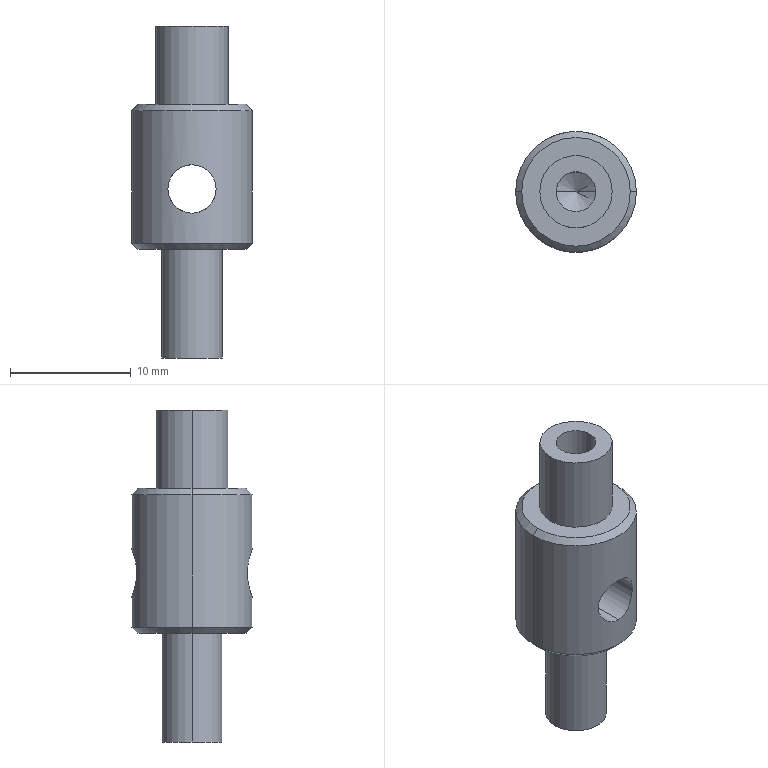Part | SolidWorks | features ICE 3, Chamfer 1, Extrusion 1, HoleWzd 1 | 1 solid | 20 faces | box 10 x 10 x 27.5 mm | volume 1083 mm3 | cylinder 10 | cone 6 | plane 4 | commonest cylinder face diameters 3.3 x2 4 x2 5 x2 6 x2 10 x2
STEP:
#1=CARTESIAN_POINT('',(-4.5,0.,0.));
#2=VERTEX_POINT('',#1);
#3=CARTESIAN_POINT('',(4.5,0.,0.));
#4=VERTEX_POINT('',#3);
#5=CARTESIAN_POINT('',(0.,0.,0.));
#6=DIRECTION('',(0.,0.,-1.));
#7=DIRECTION('',(1.,0.,0.));
#8=AXIS2_PLACEMENT_3D('',#5,#6,#7);
#9=CIRCLE('',#8,4.5);
#10=EDGE_CURVE('',#2,#4,#9,.T.);
#11=ORIENTED_EDGE('',*,*,#10,.F.);
#12=CARTESIAN_POINT('',(-5.,0.,0.5));
#13=VERTEX_POINT('',#12);
#14=CARTESIAN_POINT('',(-5.,0.,0.5));
#15=DIRECTION('',(-0.7071,0.,0.7071));
#16=VECTOR('',#15,1000.);
#17=LINE('',#14,#16);
#18=EDGE_CURVE('',#2,#13,#17,.T.);
#19=ORIENTED_EDGE('',*,*,#18,.T.);
#20=CARTESIAN_POINT('',(5.,0.,0.5));
#21=VERTEX_POINT('',#20);
#22=CARTESIAN_POINT('',(0.,0.,0.5));
#23=DIRECTION('',(0.,0.,1.));
#24=DIRECTION('',(1.,0.,0.));
#25=AXIS2_PLACEMENT_3D('',#22,#23,#24);
#26=CIRCLE('',#25,5.);
#27=EDGE_CURVE('',#21,#13,#26,.T.);
#28=ORIENTED_EDGE('',*,*,#27,.F.);
#29=CARTESIAN_POINT('',(5.,0.,0.5));
#30=DIRECTION('',(0.7071,0.,0.7071));
#31=VECTOR('',#30,1000.);
#32=LINE('',#29,#31);
#33=EDGE_CURVE('',#4,#21,#32,.T.);
#34=ORIENTED_EDGE('',*,*,#33,.F.);
#35=EDGE_LOOP('',(#11,#19,#28,#34));
#36=FACE_OUTER_BOUND('',#35,.T.);
#37=CARTESIAN_POINT('',(0.,0.,0.5));
#38=DIRECTION('',(0.,0.,1.));
#39=DIRECTION('',(1.,0.,0.));
#40=AXIS2_PLACEMENT_3D('',#37,#38,#39);
#41=CONICAL_SURFACE('',#40,5.,0.7854);
#42=ADVANCED_FACE('',(#36),#41,.T.);
#43=CARTESIAN_POINT('',(4.5,0.,12.));
#44=VERTEX_POINT('',#43);
#45=CARTESIAN_POINT('',(-4.5,0.,12.));
#46=VERTEX_POINT('',#45);
#47=CARTESIAN_POINT('',(0.,0.,12.));
#48=DIRECTION('',(0.,0.,1.));
#49=DIRECTION('',(1.,0.,0.));
#50=AXIS2_PLACEMENT_3D('',#47,#48,#49);
#51=CIRCLE('',#50,4.5);
#52=EDGE_CURVE('',#44,#46,#51,.T.);
#53=ORIENTED_EDGE('',*,*,#52,.F.);
#54=CARTESIAN_POINT('',(5.,0.,11.5));
#55=VERTEX_POINT('',#54);
#56=CARTESIAN_POINT('',(4.5,0.,12.));
#57=DIRECTION('',(0.7071,0.,-0.7071));
#58=VECTOR('',#57,1000.);
#59=LINE('',#56,#58);
#60=EDGE_CURVE('',#44,#55,#59,.T.);
#61=ORIENTED_EDGE('',*,*,#60,.T.);
#62=CARTESIAN_POINT('',(-5.,0.,11.5));
#63=VERTEX_POINT('',#62);
#64=CARTESIAN_POINT('',(0.,0.,11.5));
#65=DIRECTION('',(0.,0.,-1.));
#66=DIRECTION('',(1.,0.,0.));
#67=AXIS2_PLACEMENT_3D('',#64,#65,#66);
#68=CIRCLE('',#67,5.);
#69=EDGE_CURVE('',#63,#55,#68,.T.);
#70=ORIENTED_EDGE('',*,*,#69,.F.);
#71=CARTESIAN_POINT('',(-4.5,0.,12.));
#72=DIRECTION('',(-0.7071,0.,-0.7071));
#73=VECTOR('',#72,1000.);
#74=LINE('',#71,#73);
#75=EDGE_CURVE('',#46,#63,#74,.T.);
#76=ORIENTED_EDGE('',*,*,#75,.F.);
#77=EDGE_LOOP('',(#53,#61,#70,#76));
#78=FACE_OUTER_BOUND('',#77,.T.);
#79=CARTESIAN_POINT('',(0.,0.,12.));
#80=DIRECTION('',(0.,0.,-1.));
#81=DIRECTION('',(-1.,0.,0.));
#82=AXIS2_PLACEMENT_3D('',#79,#80,#81);
#83=CONICAL_SURFACE('',#82,4.5,0.7854);
#84=ADVANCED_FACE('',(#78),#83,.T.);
#85=CARTESIAN_POINT('',(0.,-5.,3.));
#86=VERTEX_POINT('',#85);
#87=CARTESIAN_POINT('',(0.,-5.,7.));
#88=VERTEX_POINT('',#87);
#89=CARTESIAN_POINT('',(0.,-5.,3.));
#90=CARTESIAN_POINT('',(-0.1316,-5.,3.));
#91=CARTESIAN_POINT('',(-0.2649,-4.995,3.013));
#92=CARTESIAN_POINT('',(-0.5241,-4.974,3.065));
#93=CARTESIAN_POINT('',(-0.6493,-4.959,3.104));
#94=CARTESIAN_POINT('',(-0.8912,-4.921,3.205));
#95=CARTESIAN_POINT('',(-1.008,-4.899,3.268));
#96=CARTESIAN_POINT('',(-1.223,-4.849,3.412));
#97=CARTESIAN_POINT('',(-1.323,-4.823,3.495));
#98=CARTESIAN_POINT('',(-1.507,-4.768,3.679));
#99=CARTESIAN_POINT('',(-1.589,-4.741,3.779));
#100=CARTESIAN_POINT('',(-1.733,-4.691,3.994));
#101=CARTESIAN_POINT('',(-1.796,-4.667,4.11));
#102=CARTESIAN_POINT('',(-1.896,-4.627,4.351));
#103=CARTESIAN_POINT('',(-1.935,-4.611,4.476));
#104=CARTESIAN_POINT('',(-1.987,-4.589,4.734));
#105=CARTESIAN_POINT('',(-2.,-4.583,4.868));
#106=CARTESIAN_POINT('',(-2.,-4.583,5.263));
#107=CARTESIAN_POINT('',(-1.946,-4.607,5.529));
#108=CARTESIAN_POINT('',(-1.796,-4.667,5.89));
#109=CARTESIAN_POINT('',(-1.733,-4.691,6.006));
#110=CARTESIAN_POINT('',(-1.589,-4.742,6.222));
#111=CARTESIAN_POINT('',(-1.507,-4.769,6.322));
#112=CARTESIAN_POINT('',(-1.323,-4.823,6.505));
#113=CARTESIAN_POINT('',(-1.222,-4.85,6.589));
#114=CARTESIAN_POINT('',(-1.007,-4.899,6.733));
#115=CARTESIAN_POINT('',(-0.8926,-4.921,6.795));
#116=CARTESIAN_POINT('',(-0.5273,-4.978,6.947));
#117=CARTESIAN_POINT('',(-0.2671,-5.,7.));
#118=CARTESIAN_POINT('',(0.,-5.,7.));
#119=B_SPLINE_CURVE_WITH_KNOTS('',3,(#89,#90,#91,#92,#93,#94,#95,#96,#97,#98,#99,#100,#101,#102,#103,#104,#105,#106,#107,#108,#109,#110,#111,#112,#113,#114,#115,#116,#117,#118),.UNSPECIFIED.,.F.,.F.,(4,2,2,2,2,2,2,2,2,2,2,2,2,2,4),(0.00632,0.006715,0.007109,0.007504,0.007899,0.008293,0.008688,0.009083,0.009478,0.01027,0.01066,0.01106,0.01145,0.01185,0.01264),.UNSPECIFIED.);
#120=EDGE_CURVE('',#86,#88,#119,.T.);
#121=ORIENTED_EDGE('',*,*,#120,.F.);
#122=CARTESIAN_POINT('',(0.,5.,3.));
#123=VERTEX_POINT('',#122);
#124=CARTESIAN_POINT('',(0.,-7.5,3.));
#125=DIRECTION('',(0.,1.,0.));
#126=VECTOR('',#125,1000.);
#127=LINE('',#124,#126);
#128=EDGE_CURVE('',#86,#123,#127,.T.);
#129=ORIENTED_EDGE('',*,*,#128,.T.);
#130=CARTESIAN_POINT('',(0.,5.,7.));
#131=VERTEX_POINT('',#130);
#132=CARTESIAN_POINT('',(0.,5.,7.));
#133=CARTESIAN_POINT('',(-0.1337,5.,7.));
#134=CARTESIAN_POINT('',(-0.2648,4.995,6.987));
#135=CARTESIAN_POINT('',(-0.5224,4.974,6.935));
#136=CARTESIAN_POINT('',(-0.6502,4.959,6.896));
#137=CARTESIAN_POINT('',(-0.8919,4.921,6.795));
#138=CARTESIAN_POINT('',(-1.006,4.899,6.733));
#139=CARTESIAN_POINT('',(-1.223,4.849,6.588));
#140=CARTESIAN_POINT('',(-1.324,4.822,6.505));
#141=CARTESIAN_POINT('',(-1.597,4.742,6.231));
#142=CARTESIAN_POINT('',(-1.746,4.687,6.01));
#143=CARTESIAN_POINT('',(-1.896,4.627,5.65));
#144=CARTESIAN_POINT('',(-1.935,4.61,5.523));
#145=CARTESIAN_POINT('',(-1.987,4.588,5.264));
#146=CARTESIAN_POINT('',(-2.,4.583,5.133));
#147=CARTESIAN_POINT('',(-2.,4.583,4.869));
#148=CARTESIAN_POINT('',(-1.987,4.588,4.735));
#149=CARTESIAN_POINT('',(-1.935,4.611,4.477));
#150=CARTESIAN_POINT('',(-1.897,4.627,4.352));
#151=CARTESIAN_POINT('',(-1.795,4.667,4.108));
#152=CARTESIAN_POINT('',(-1.733,4.691,3.994));
#153=CARTESIAN_POINT('',(-1.589,4.741,3.778));
#154=CARTESIAN_POINT('',(-1.505,4.769,3.677));
#155=CARTESIAN_POINT('',(-1.322,4.823,3.494));
#156=CARTESIAN_POINT('',(-1.223,4.85,3.412));
#157=CARTESIAN_POINT('',(-1.006,4.899,3.267));
#158=CARTESIAN_POINT('',(-0.8898,4.922,3.204));
#159=CARTESIAN_POINT('',(-0.5291,4.978,3.054));
#160=CARTESIAN_POINT('',(-0.2633,5.,3.));
#161=CARTESIAN_POINT('',(0.,5.,3.));
#162=B_SPLINE_CURVE_WITH_KNOTS('',3,(#132,#133,#134,#135,#136,#137,#138,#139,#140,#141,#142,#143,#144,#145,#146,#147,#148,#149,#150,#151,#152,#153,#154,#155,#156,#157,#158,#159,#160,#161),.UNSPECIFIED.,.F.,.F.,(4,2,2,2,2,2,2,2,2,2,2,2,2,2,4),(0.,0.000395,0.00079,0.001185,0.00158,0.00237,0.002765,0.00316,0.003555,0.00395,0.004345,0.00474,0.005135,0.00553,0.00632),.UNSPECIFIED.);
#163=EDGE_CURVE('',#131,#123,#162,.T.);
#164=ORIENTED_EDGE('',*,*,#163,.F.);
#165=CARTESIAN_POINT('',(0.,-7.5,7.));
#166=DIRECTION('',(0.,1.,0.));
#167=VECTOR('',#166,1000.);
#168=LINE('',#165,#167);
#169=EDGE_CURVE('',#88,#131,#168,.T.);
#170=ORIENTED_EDGE('',*,*,#169,.F.);
#171=EDGE_LOOP('',(#121,#129,#164,#170));
#172=FACE_OUTER_BOUND('',#171,.T.);
#173=CARTESIAN_POINT('',(0.,-7.5,5.));
#174=DIRECTION('',(0.,1.,0.));
#175=DIRECTION('',(0.,0.,1.));
#176=AXIS2_PLACEMENT_3D('',#173,#174,#175);
#177=CYLINDRICAL_SURFACE('',#176,2.);
#178=ADVANCED_FACE('',(#172),#177,.F.);
#179=CARTESIAN_POINT('',(-2.5,0.,-9.));
#180=VERTEX_POINT('',#179);
#181=CARTESIAN_POINT('',(2.5,0.,-9.));
#182=VERTEX_POINT('',#181);
#183=CARTESIAN_POINT('',(0.,0.,-9.));
#184=DIRECTION('',(0.,0.,-1.));
#185=DIRECTION('',(-1.,0.,0.));
#186=AXIS2_PLACEMENT_3D('',#183,#184,#185);
#187=CIRCLE('',#186,2.5);
#188=EDGE_CURVE('',#180,#182,#187,.T.);
#189=ORIENTED_EDGE('',*,*,#188,.F.);
#190=CARTESIAN_POINT('',(-2.5,0.,0.));
#191=VERTEX_POINT('',#190);
#192=CARTESIAN_POINT('',(-2.5,0.,-9.));
#193=DIRECTION('',(0.,0.,1.));
#194=VECTOR('',#193,1000.);
#195=LINE('',#192,#194);
#196=EDGE_CURVE('',#180,#191,#195,.T.);
#197=ORIENTED_EDGE('',*,*,#196,.T.);
#198=CARTESIAN_POINT('',(2.5,0.,0.));
#199=VERTEX_POINT('',#198);
#200=CARTESIAN_POINT('',(0.,0.,0.));
#201=DIRECTION('',(0.,0.,-1.));
#202=DIRECTION('',(1.,0.,0.));
#203=AXIS2_PLACEMENT_3D('',#200,#201,#202);
#204=CIRCLE('',#203,2.5);
#205=EDGE_CURVE('',#191,#199,#204,.T.);
#206=ORIENTED_EDGE('',*,*,#205,.T.);
#207=CARTESIAN_POINT('',(2.5,0.,-9.));
#208=DIRECTION('',(0.,0.,1.));
#209=VECTOR('',#208,1000.);
#210=LINE('',#207,#209);
#211=EDGE_CURVE('',#182,#199,#210,.T.);
#212=ORIENTED_EDGE('',*,*,#211,.F.);
#213=EDGE_LOOP('',(#189,#197,#206,#212));
#214=FACE_OUTER_BOUND('',#213,.T.);
#215=CARTESIAN_POINT('',(0.,0.,-9.));
#216=DIRECTION('',(0.,0.,1.));
#217=DIRECTION('',(1.,0.,0.));
#218=AXIS2_PLACEMENT_3D('',#215,#216,#217);
#219=CYLINDRICAL_SURFACE('',#218,2.5);
#220=ADVANCED_FACE('',(#214),#219,.T.);
#221=CARTESIAN_POINT('',(-1.65,0.,8.4));
#222=VERTEX_POINT('',#221);
#223=CARTESIAN_POINT('',(1.65,0.,8.4));
#224=VERTEX_POINT('',#223);
#225=CARTESIAN_POINT('',(0.,0.,8.4));
#226=DIRECTION('',(0.,0.,1.));
#227=DIRECTION('',(1.,0.,0.));
#228=AXIS2_PLACEMENT_3D('',#225,#226,#227);
#229=CIRCLE('',#228,1.65);
#230=EDGE_CURVE('',#222,#224,#229,.T.);
#231=ORIENTED_EDGE('',*,*,#230,.F.);
#232=CARTESIAN_POINT('',(-1.65,0.,18.5));
#233=VERTEX_POINT('',#232);
#234=CARTESIAN_POINT('',(-1.65,0.,18.5));
#235=DIRECTION('',(0.,0.,1.));
#236=VECTOR('',#235,1000.);
#237=LINE('',#234,#236);
#238=EDGE_CURVE('',#222,#233,#237,.T.);
#239=ORIENTED_EDGE('',*,*,#238,.T.);
#240=CARTESIAN_POINT('',(1.65,0.,18.5));
#241=VERTEX_POINT('',#240);
#242=CARTESIAN_POINT('',(0.,0.,18.5));
#243=DIRECTION('',(0.,0.,1.));
#244=DIRECTION('',(1.,0.,0.));
#245=AXIS2_PLACEMENT_3D('',#242,#243,#244);
#246=CIRCLE('',#245,1.65);
#247=EDGE_CURVE('',#233,#241,#246,.T.);
#248=ORIENTED_EDGE('',*,*,#247,.T.);
#249=CARTESIAN_POINT('',(1.65,0.,18.5));
#250=DIRECTION('',(0.,0.,1.));
#251=VECTOR('',#250,1000.);
#252=LINE('',#249,#251);
#253=EDGE_CURVE('',#224,#241,#252,.T.);
#254=ORIENTED_EDGE('',*,*,#253,.F.);
#255=EDGE_LOOP('',(#231,#239,#248,#254));
#256=FACE_OUTER_BOUND('',#255,.T.);
#257=CARTESIAN_POINT('',(0.,0.,18.5));
#258=DIRECTION('',(0.,0.,1.));
#259=DIRECTION('',(1.,0.,0.));
#260=AXIS2_PLACEMENT_3D('',#257,#258,#259);
#261=CYLINDRICAL_SURFACE('',#260,1.65);
#262=ADVANCED_FACE('',(#256),#261,.F.);
#263=CARTESIAN_POINT('',(0.,0.,7.409));
#264=VERTEX_POINT('',#263);
#265=CARTESIAN_POINT('',(1.65,0.,8.4));
#266=DIRECTION('',(0.8572,0.,0.515));
#267=VECTOR('',#266,1000.);
#268=LINE('',#265,#267);
#269=EDGE_CURVE('',#264,#224,#268,.T.);
#270=ORIENTED_EDGE('',*,*,#269,.F.);
#271=CARTESIAN_POINT('',(-1.65,0.,8.4));
#272=DIRECTION('',(-0.8572,0.,0.515));
#273=VECTOR('',#272,1000.);
#274=LINE('',#271,#273);
#275=EDGE_CURVE('',#264,#222,#274,.T.);
#276=ORIENTED_EDGE('',*,*,#275,.T.);
#277=ORIENTED_EDGE('',*,*,#230,.T.);
#278=EDGE_LOOP('',(#270,#276,#277));
#279=FACE_OUTER_BOUND('',#278,.T.);
#280=CARTESIAN_POINT('',(0.,0.,8.4));
#281=DIRECTION('',(0.,0.,1.));
#282=DIRECTION('',(1.,0.,0.));
#283=AXIS2_PLACEMENT_3D('',#280,#281,#282);
#284=CONICAL_SURFACE('',#283,1.65,1.03);
#285=ADVANCED_FACE('',(#279),#284,.F.);
#286=CARTESIAN_POINT('',(3.,0.,18.5));
#287=VERTEX_POINT('',#286);
#288=CARTESIAN_POINT('',(-3.,0.,18.5));
#289=VERTEX_POINT('',#288);
#290=CARTESIAN_POINT('',(0.,0.,18.5));
#291=DIRECTION('',(0.,0.,1.));
#292=DIRECTION('',(1.,0.,0.));
#293=AXIS2_PLACEMENT_3D('',#290,#291,#292);
#294=CIRCLE('',#293,3.);
#295=EDGE_CURVE('',#287,#289,#294,.T.);
#296=ORIENTED_EDGE('',*,*,#295,.F.);
#297=CARTESIAN_POINT('',(3.,0.,12.));
#298=VERTEX_POINT('',#297);
#299=CARTESIAN_POINT('',(3.,0.,18.5));
#300=DIRECTION('',(0.,0.,-1.));
#301=VECTOR('',#300,1000.);
#302=LINE('',#299,#301);
#303=EDGE_CURVE('',#287,#298,#302,.T.);
#304=ORIENTED_EDGE('',*,*,#303,.T.);
#305=CARTESIAN_POINT('',(-3.,0.,12.));
#306=VERTEX_POINT('',#305);
#307=CARTESIAN_POINT('',(0.,0.,12.));
#308=DIRECTION('',(0.,0.,1.));
#309=DIRECTION('',(1.,0.,0.));
#310=AXIS2_PLACEMENT_3D('',#307,#308,#309);
#311=CIRCLE('',#310,3.);
#312=EDGE_CURVE('',#298,#306,#311,.T.);
#313=ORIENTED_EDGE('',*,*,#312,.T.);
#314=CARTESIAN_POINT('',(-3.,0.,18.5));
#315=DIRECTION('',(0.,0.,-1.));
#316=VECTOR('',#315,1000.);
#317=LINE('',#314,#316);
#318=EDGE_CURVE('',#289,#306,#317,.T.);
#319=ORIENTED_EDGE('',*,*,#318,.F.);
#320=EDGE_LOOP('',(#296,#304,#313,#319));
#321=FACE_OUTER_BOUND('',#320,.T.);
#322=CARTESIAN_POINT('',(0.,0.,18.5));
#323=DIRECTION('',(0.,0.,-1.));
#324=DIRECTION('',(-1.,0.,0.));
#325=AXIS2_PLACEMENT_3D('',#322,#323,#324);
#326=CYLINDRICAL_SURFACE('',#325,3.);
#327=ADVANCED_FACE('',(#321),#326,.T.);
#328=ORIENTED_EDGE('',*,*,#163,.T.);
#329=CARTESIAN_POINT('',(0.,5.,3.));
#330=CARTESIAN_POINT('',(0.1316,5.,3.));
#331=CARTESIAN_POINT('',(0.2649,4.995,3.013));
#332=CARTESIAN_POINT('',(0.5241,4.974,3.065));
#333=CARTESIAN_POINT('',(0.6493,4.959,3.104));
#334=CARTESIAN_POINT('',(0.8912,4.921,3.205));
#335=CARTESIAN_POINT('',(1.008,4.899,3.268));
#336=CARTESIAN_POINT('',(1.223,4.849,3.412));
#337=CARTESIAN_POINT('',(1.323,4.823,3.495));
#338=CARTESIAN_POINT('',(1.507,4.768,3.679));
#339=CARTESIAN_POINT('',(1.589,4.741,3.779));
#340=CARTESIAN_POINT('',(1.733,4.691,3.994));
#341=CARTESIAN_POINT('',(1.796,4.667,4.11));
#342=CARTESIAN_POINT('',(1.896,4.627,4.351));
#343=CARTESIAN_POINT('',(1.935,4.611,4.476));
#344=CARTESIAN_POINT('',(1.987,4.589,4.734));
#345=CARTESIAN_POINT('',(2.,4.583,4.868));
#346=CARTESIAN_POINT('',(2.,4.583,5.263));
#347=CARTESIAN_POINT('',(1.946,4.607,5.529));
#348=CARTESIAN_POINT('',(1.796,4.667,5.89));
#349=CARTESIAN_POINT('',(1.733,4.691,6.006));
#350=CARTESIAN_POINT('',(1.589,4.742,6.222));
#351=CARTESIAN_POINT('',(1.507,4.769,6.322));
#352=CARTESIAN_POINT('',(1.323,4.823,6.505));
#353=CARTESIAN_POINT('',(1.222,4.85,6.589));
#354=CARTESIAN_POINT('',(1.007,4.899,6.733));
#355=CARTESIAN_POINT('',(0.8926,4.921,6.795));
#356=CARTESIAN_POINT('',(0.5273,4.978,6.947));
#357=CARTESIAN_POINT('',(0.2671,5.,7.));
#358=CARTESIAN_POINT('',(0.,5.,7.));
#359=B_SPLINE_CURVE_WITH_KNOTS('',3,(#329,#330,#331,#332,#333,#334,#335,#336,#337,#338,#339,#340,#341,#342,#343,#344,#345,#346,#347,#348,#349,#350,#351,#352,#353,#354,#355,#356,#357,#358),.UNSPECIFIED.,.F.,.F.,(4,2,2,2,2,2,2,2,2,2,2,2,2,2,4),(0.00632,0.006715,0.007109,0.007504,0.007899,0.008293,0.008688,0.009083,0.009478,0.01027,0.01066,0.01106,0.01145,0.01185,0.01264),.UNSPECIFIED.);
#360=EDGE_CURVE('',#123,#131,#359,.T.);
#361=ORIENTED_EDGE('',*,*,#360,.T.);
#362=EDGE_LOOP('',(#328,#361));
#363=FACE_BOUND('',#362,.T.);
#364=ORIENTED_EDGE('',*,*,#69,.T.);
#365=CARTESIAN_POINT('',(5.,0.,12.));
#366=DIRECTION('',(0.,0.,-1.));
#367=VECTOR('',#366,1000.);
#368=LINE('',#365,#367);
#369=EDGE_CURVE('',#55,#21,#368,.T.);
#370=ORIENTED_EDGE('',*,*,#369,.T.);
#371=ORIENTED_EDGE('',*,*,#27,.T.);
#372=CARTESIAN_POINT('',(-5.,0.,12.));
#373=DIRECTION('',(0.,0.,-1.));
#374=VECTOR('',#373,1000.);
#375=LINE('',#372,#374);
#376=EDGE_CURVE('',#63,#13,#375,.T.);
#377=ORIENTED_EDGE('',*,*,#376,.F.);
#378=EDGE_LOOP('',(#364,#370,#371,#377));
#379=FACE_OUTER_BOUND('',#378,.T.);
#380=CARTESIAN_POINT('',(0.,0.,12.));
#381=DIRECTION('',(0.,0.,-1.));
#382=DIRECTION('',(-1.,0.,0.));
#383=AXIS2_PLACEMENT_3D('',#380,#381,#382);
#384=CYLINDRICAL_SURFACE('',#383,5.);
#385=ADVANCED_FACE('',(#363,#379),#384,.T.);
#386=CARTESIAN_POINT('',(0.,0.,0.));
#387=DIRECTION('',(0.,0.,-1.));
#388=DIRECTION('',(1.,0.,0.));
#389=AXIS2_PLACEMENT_3D('',#386,#387,#388);
#390=CIRCLE('',#389,4.5);
#391=EDGE_CURVE('',#4,#2,#390,.T.);
#392=ORIENTED_EDGE('',*,*,#391,.T.);
#393=ORIENTED_EDGE('',*,*,#10,.T.);
#394=EDGE_LOOP('',(#392,#393));
#395=FACE_OUTER_BOUND('',#394,.T.);
#396=CARTESIAN_POINT('',(0.,0.,0.));
#397=DIRECTION('',(0.,0.,-1.));
#398=DIRECTION('',(1.,0.,0.));
#399=AXIS2_PLACEMENT_3D('',#396,#397,#398);
#400=CIRCLE('',#399,2.5);
#401=EDGE_CURVE('',#199,#191,#400,.T.);
#402=ORIENTED_EDGE('',*,*,#401,.F.);
#403=ORIENTED_EDGE('',*,*,#205,.F.);
#404=EDGE_LOOP('',(#402,#403));
#405=FACE_BOUND('',#404,.T.);
#406=CARTESIAN_POINT('',(0.,0.,0.));
#407=DIRECTION('',(0.,0.,1.));
#408=DIRECTION('',(1.,0.,0.));
#409=AXIS2_PLACEMENT_3D('',#406,#407,#408);
#410=PLANE('',#409);
#411=ADVANCED_FACE('',(#395,#405),#410,.F.);
#412=CARTESIAN_POINT('',(0.,0.,12.));
#413=DIRECTION('',(0.,0.,1.));
#414=DIRECTION('',(1.,0.,0.));
#415=AXIS2_PLACEMENT_3D('',#412,#413,#414);
#416=CIRCLE('',#415,4.5);
#417=EDGE_CURVE('',#46,#44,#416,.T.);
#418=ORIENTED_EDGE('',*,*,#417,.T.);
#419=ORIENTED_EDGE('',*,*,#52,.T.);
#420=EDGE_LOOP('',(#418,#419));
#421=FACE_OUTER_BOUND('',#420,.T.);
#422=CARTESIAN_POINT('',(0.,0.,12.));
#423=DIRECTION('',(0.,0.,1.));
#424=DIRECTION('',(1.,0.,0.));
#425=AXIS2_PLACEMENT_3D('',#422,#423,#424);
#426=CIRCLE('',#425,3.);
#427=EDGE_CURVE('',#306,#298,#426,.T.);
#428=ORIENTED_EDGE('',*,*,#427,.F.);
#429=ORIENTED_EDGE('',*,*,#312,.F.);
#430=EDGE_LOOP('',(#428,#429));
#431=FACE_BOUND('',#430,.T.);
#432=CARTESIAN_POINT('',(0.,0.,12.));
#433=DIRECTION('',(0.,0.,1.));
#434=DIRECTION('',(1.,0.,0.));
#435=AXIS2_PLACEMENT_3D('',#432,#433,#434);
#436=PLANE('',#435);
#437=ADVANCED_FACE('',(#421,#431),#436,.T.);
#438=ORIENTED_EDGE('',*,*,#369,.F.);
#439=CARTESIAN_POINT('',(0.,0.,11.5));
#440=DIRECTION('',(0.,0.,-1.));
#441=DIRECTION('',(1.,0.,0.));
#442=AXIS2_PLACEMENT_3D('',#439,#440,#441);
#443=CIRCLE('',#442,5.);
#444=EDGE_CURVE('',#55,#63,#443,.T.);
#445=ORIENTED_EDGE('',*,*,#444,.T.);
#446=ORIENTED_EDGE('',*,*,#376,.T.);
#447=CARTESIAN_POINT('',(0.,0.,0.5));
#448=DIRECTION('',(0.,0.,1.));
#449=DIRECTION('',(1.,0.,0.));
#450=AXIS2_PLACEMENT_3D('',#447,#448,#449);
#451=CIRCLE('',#450,5.);
#452=EDGE_CURVE('',#13,#21,#451,.T.);
#453=ORIENTED_EDGE('',*,*,#452,.T.);
#454=EDGE_LOOP('',(#438,#445,#446,#453));
#455=FACE_OUTER_BOUND('',#454,.T.);
#456=CARTESIAN_POINT('',(0.,-5.,7.));
#457=CARTESIAN_POINT('',(0.1337,-5.,7.));
#458=CARTESIAN_POINT('',(0.2648,-4.995,6.987));
#459=CARTESIAN_POINT('',(0.5224,-4.974,6.935));
#460=CARTESIAN_POINT('',(0.6502,-4.959,6.896));
#461=CARTESIAN_POINT('',(0.8919,-4.921,6.795));
#462=CARTESIAN_POINT('',(1.006,-4.899,6.733));
#463=CARTESIAN_POINT('',(1.223,-4.849,6.588));
#464=CARTESIAN_POINT('',(1.324,-4.822,6.505));
#465=CARTESIAN_POINT('',(1.597,-4.742,6.231));
#466=CARTESIAN_POINT('',(1.746,-4.687,6.01));
#467=CARTESIAN_POINT('',(1.896,-4.627,5.65));
#468=CARTESIAN_POINT('',(1.935,-4.61,5.523));
#469=CARTESIAN_POINT('',(1.987,-4.588,5.264));
#470=CARTESIAN_POINT('',(2.,-4.583,5.133));
#471=CARTESIAN_POINT('',(2.,-4.583,4.869));
#472=CARTESIAN_POINT('',(1.987,-4.588,4.735));
#473=CARTESIAN_POINT('',(1.935,-4.611,4.477));
#474=CARTESIAN_POINT('',(1.897,-4.627,4.352));
#475=CARTESIAN_POINT('',(1.795,-4.667,4.108));
#476=CARTESIAN_POINT('',(1.733,-4.691,3.994));
#477=CARTESIAN_POINT('',(1.589,-4.741,3.778));
#478=CARTESIAN_POINT('',(1.505,-4.769,3.677));
#479=CARTESIAN_POINT('',(1.322,-4.823,3.494));
#480=CARTESIAN_POINT('',(1.223,-4.85,3.412));
#481=CARTESIAN_POINT('',(1.006,-4.899,3.267));
#482=CARTESIAN_POINT('',(0.8898,-4.922,3.204));
#483=CARTESIAN_POINT('',(0.5291,-4.978,3.054));
#484=CARTESIAN_POINT('',(0.2633,-5.,3.));
#485=CARTESIAN_POINT('',(0.,-5.,3.));
#486=B_SPLINE_CURVE_WITH_KNOTS('',3,(#456,#457,#458,#459,#460,#461,#462,#463,#464,#465,#466,#467,#468,#469,#470,#471,#472,#473,#474,#475,#476,#477,#478,#479,#480,#481,#482,#483,#484,#485),.UNSPECIFIED.,.F.,.F.,(4,2,2,2,2,2,2,2,2,2,2,2,2,2,4),(0.,0.000395,0.00079,0.001185,0.00158,0.00237,0.002765,0.00316,0.003555,0.00395,0.004345,0.00474,0.005135,0.00553,0.00632),.UNSPECIFIED.);
#487=EDGE_CURVE('',#88,#86,#486,.T.);
#488=ORIENTED_EDGE('',*,*,#487,.T.);
#489=ORIENTED_EDGE('',*,*,#120,.T.);
#490=EDGE_LOOP('',(#488,#489));
#491=FACE_BOUND('',#490,.T.);
#492=CARTESIAN_POINT('',(0.,0.,12.));
#493=DIRECTION('',(0.,0.,-1.));
#494=DIRECTION('',(-1.,0.,0.));
#495=AXIS2_PLACEMENT_3D('',#492,#493,#494);
#496=CYLINDRICAL_SURFACE('',#495,5.);
#497=ADVANCED_FACE('',(#455,#491),#496,.T.);
#498=ORIENTED_EDGE('',*,*,#303,.F.);
#499=CARTESIAN_POINT('',(0.,0.,18.5));
#500=DIRECTION('',(0.,0.,1.));
#501=DIRECTION('',(1.,0.,0.));
#502=AXIS2_PLACEMENT_3D('',#499,#500,#501);
#503=CIRCLE('',#502,3.);
#504=EDGE_CURVE('',#289,#287,#503,.T.);
#505=ORIENTED_EDGE('',*,*,#504,.F.);
#506=ORIENTED_EDGE('',*,*,#318,.T.);
#507=ORIENTED_EDGE('',*,*,#427,.T.);
#508=EDGE_LOOP('',(#498,#505,#506,#507));
#509=FACE_OUTER_BOUND('',#508,.T.);
#510=CARTESIAN_POINT('',(0.,0.,18.5));
#511=DIRECTION('',(0.,0.,-1.));
#512=DIRECTION('',(-1.,0.,0.));
#513=AXIS2_PLACEMENT_3D('',#510,#511,#512);
#514=CYLINDRICAL_SURFACE('',#513,3.);
#515=ADVANCED_FACE('',(#509),#514,.T.);
#516=CARTESIAN_POINT('',(0.,0.,18.5));
#517=DIRECTION('',(0.,0.,1.));
#518=DIRECTION('',(1.,0.,0.));
#519=AXIS2_PLACEMENT_3D('',#516,#517,#518);
#520=CIRCLE('',#519,1.65);
#521=EDGE_CURVE('',#241,#233,#520,.T.);
#522=ORIENTED_EDGE('',*,*,#521,.F.);
#523=ORIENTED_EDGE('',*,*,#247,.F.);
#524=EDGE_LOOP('',(#522,#523));
#525=FACE_BOUND('',#524,.T.);
#526=ORIENTED_EDGE('',*,*,#504,.T.);
#527=ORIENTED_EDGE('',*,*,#295,.T.);
#528=EDGE_LOOP('',(#526,#527));
#529=FACE_OUTER_BOUND('',#528,.T.);
#530=CARTESIAN_POINT('',(0.,0.,18.5));
#531=DIRECTION('',(0.,0.,1.));
#532=DIRECTION('',(1.,0.,0.));
#533=AXIS2_PLACEMENT_3D('',#530,#531,#532);
#534=PLANE('',#533);
#535=ADVANCED_FACE('',(#525,#529),#534,.T.);
#536=ORIENTED_EDGE('',*,*,#275,.F.);
#537=ORIENTED_EDGE('',*,*,#269,.T.);
#538=CARTESIAN_POINT('',(0.,0.,8.4));
#539=DIRECTION('',(0.,0.,1.));
#540=DIRECTION('',(1.,0.,0.));
#541=AXIS2_PLACEMENT_3D('',#538,#539,#540);
#542=CIRCLE('',#541,1.65);
#543=EDGE_CURVE('',#224,#222,#542,.T.);
#544=ORIENTED_EDGE('',*,*,#543,.T.);
#545=EDGE_LOOP('',(#536,#537,#544));
#546=FACE_OUTER_BOUND('',#545,.T.);
#547=CARTESIAN_POINT('',(0.,0.,8.4));
#548=DIRECTION('',(0.,0.,1.));
#549=DIRECTION('',(1.,0.,0.));
#550=AXIS2_PLACEMENT_3D('',#547,#548,#549);
#551=CONICAL_SURFACE('',#550,1.65,1.03);
#552=ADVANCED_FACE('',(#546),#551,.F.);
#553=ORIENTED_EDGE('',*,*,#238,.F.);
#554=ORIENTED_EDGE('',*,*,#543,.F.);
#555=ORIENTED_EDGE('',*,*,#253,.T.);
#556=ORIENTED_EDGE('',*,*,#521,.T.);
#557=EDGE_LOOP('',(#553,#554,#555,#556));
#558=FACE_OUTER_BOUND('',#557,.T.);
#559=CARTESIAN_POINT('',(0.,0.,18.5));
#560=DIRECTION('',(0.,0.,1.));
#561=DIRECTION('',(1.,0.,0.));
#562=AXIS2_PLACEMENT_3D('',#559,#560,#561);
#563=CYLINDRICAL_SURFACE('',#562,1.65);
#564=ADVANCED_FACE('',(#558),#563,.F.);
#565=ORIENTED_EDGE('',*,*,#196,.F.);
#566=CARTESIAN_POINT('',(0.,0.,-9.));
#567=DIRECTION('',(0.,0.,-1.));
#568=DIRECTION('',(-1.,0.,0.));
#569=AXIS2_PLACEMENT_3D('',#566,#567,#568);
#570=CIRCLE('',#569,2.5);
#571=EDGE_CURVE('',#182,#180,#570,.T.);
#572=ORIENTED_EDGE('',*,*,#571,.F.);
#573=ORIENTED_EDGE('',*,*,#211,.T.);
#574=ORIENTED_EDGE('',*,*,#401,.T.);
#575=EDGE_LOOP('',(#565,#572,#573,#574));
#576=FACE_OUTER_BOUND('',#575,.T.);
#577=CARTESIAN_POINT('',(0.,0.,-9.));
#578=DIRECTION('',(0.,0.,1.));
#579=DIRECTION('',(1.,0.,0.));
#580=AXIS2_PLACEMENT_3D('',#577,#578,#579);
#581=CYLINDRICAL_SURFACE('',#580,2.5);
#582=ADVANCED_FACE('',(#576),#581,.T.);
#583=ORIENTED_EDGE('',*,*,#571,.T.);
#584=ORIENTED_EDGE('',*,*,#188,.T.);
#585=EDGE_LOOP('',(#583,#584));
#586=FACE_OUTER_BOUND('',#585,.T.);
#587=CARTESIAN_POINT('',(0.,0.,-9.));
#588=DIRECTION('',(0.,0.,-1.));
#589=DIRECTION('',(-1.,0.,0.));
#590=AXIS2_PLACEMENT_3D('',#587,#588,#589);
#591=PLANE('',#590);
#592=ADVANCED_FACE('',(#586),#591,.T.);
#593=ORIENTED_EDGE('',*,*,#128,.F.);
#594=ORIENTED_EDGE('',*,*,#487,.F.);
#595=ORIENTED_EDGE('',*,*,#169,.T.);
#596=ORIENTED_EDGE('',*,*,#360,.F.);
#597=EDGE_LOOP('',(#593,#594,#595,#596));
#598=FACE_OUTER_BOUND('',#597,.T.);
#599=CARTESIAN_POINT('',(0.,-7.5,5.));
#600=DIRECTION('',(0.,1.,0.));
#601=DIRECTION('',(0.,0.,1.));
#602=AXIS2_PLACEMENT_3D('',#599,#600,#601);
#603=CYLINDRICAL_SURFACE('',#602,2.);
#604=ADVANCED_FACE('',(#598),#603,.F.);
#605=ORIENTED_EDGE('',*,*,#60,.F.);
#606=ORIENTED_EDGE('',*,*,#417,.F.);
#607=ORIENTED_EDGE('',*,*,#75,.T.);
#608=ORIENTED_EDGE('',*,*,#444,.F.);
#609=EDGE_LOOP('',(#605,#606,#607,#608));
#610=FACE_OUTER_BOUND('',#609,.T.);
#611=CARTESIAN_POINT('',(0.,0.,12.));
#612=DIRECTION('',(0.,0.,-1.));
#613=DIRECTION('',(-1.,0.,0.));
#614=AXIS2_PLACEMENT_3D('',#611,#612,#613);
#615=CONICAL_SURFACE('',#614,4.5,0.7854);
#616=ADVANCED_FACE('',(#610),#615,.T.);
#617=ORIENTED_EDGE('',*,*,#18,.F.);
#618=ORIENTED_EDGE('',*,*,#391,.F.);
#619=ORIENTED_EDGE('',*,*,#33,.T.);
#620=ORIENTED_EDGE('',*,*,#452,.F.);
#621=EDGE_LOOP('',(#617,#618,#619,#620));
#622=FACE_OUTER_BOUND('',#621,.T.);
#623=CARTESIAN_POINT('',(0.,0.,0.5));
#624=DIRECTION('',(0.,0.,1.));
#625=DIRECTION('',(1.,0.,0.));
#626=AXIS2_PLACEMENT_3D('',#623,#624,#625);
#627=CONICAL_SURFACE('',#626,5.,0.7854);
#628=ADVANCED_FACE('',(#622),#627,.T.);
#629=CLOSED_SHELL('',(#42,#84,#178,#220,#262,#285,#327,#385,#411,#437,#497,#515,#535,#552,#564,#582,#592,#604,#616,#628));
#630=MANIFOLD_SOLID_BREP('',#629);
#631=CARTESIAN_POINT('',(0.,0.,0.));
#632=DIRECTION('',(0.,0.,1.));
#633=DIRECTION('',(1.,0.,0.));
#634=AXIS2_PLACEMENT_3D('',#631,#632,#633);
#635=(LENGTH_UNIT()NAMED_UNIT(*)SI_UNIT(.MILLI.,.METRE.));
#636=UNCERTAINTY_MEASURE_WITH_UNIT(LENGTH_MEASURE(0.00001),#635,'','');
#637=(NAMED_UNIT(*)PLANE_ANGLE_UNIT()SI_UNIT($,.RADIAN.));
#638=(NAMED_UNIT(*)SI_UNIT($,.STERADIAN.)SOLID_ANGLE_UNIT());
#639=(GEOMETRIC_REPRESENTATION_CONTEXT(3)GLOBAL_UNCERTAINTY_ASSIGNED_CONTEXT((#636))GLOBAL_UNIT_ASSIGNED_CONTEXT((#635,#637,#638))REPRESENTATION_CONTEXT('',''));
#640=ADVANCED_BREP_SHAPE_REPRESENTATION('',(#630,#634),#639);